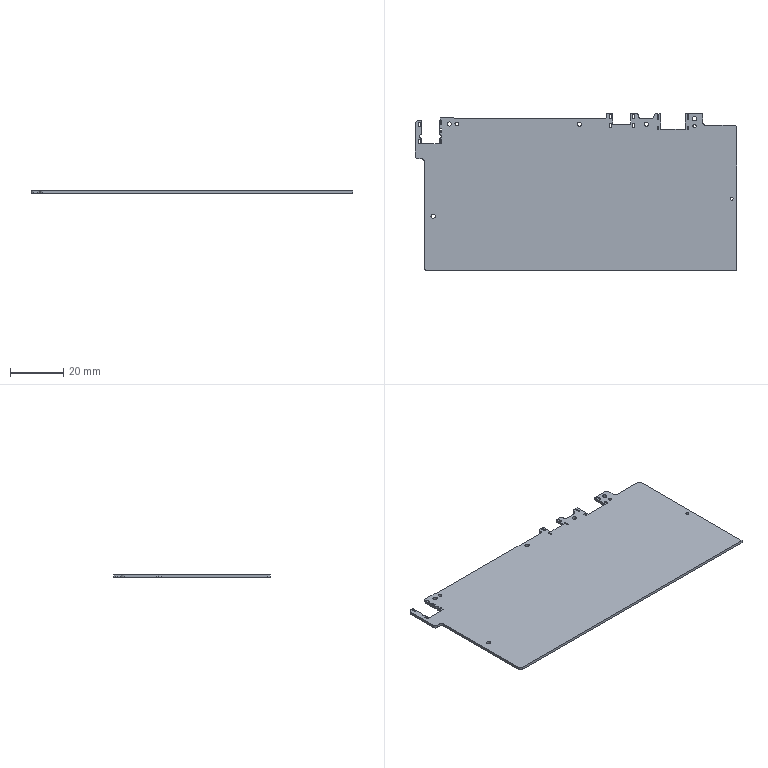Part | Creo | 1 solid | 116 faces | box 121 x 59 x 1 mm | volume 6613 mm3 | cylinder 59 | plane 57 | commonest cylinder face diameters 0.6 x18 1.6 x11 2 x9 0.66 x8 1.3 x6 1.2 x3